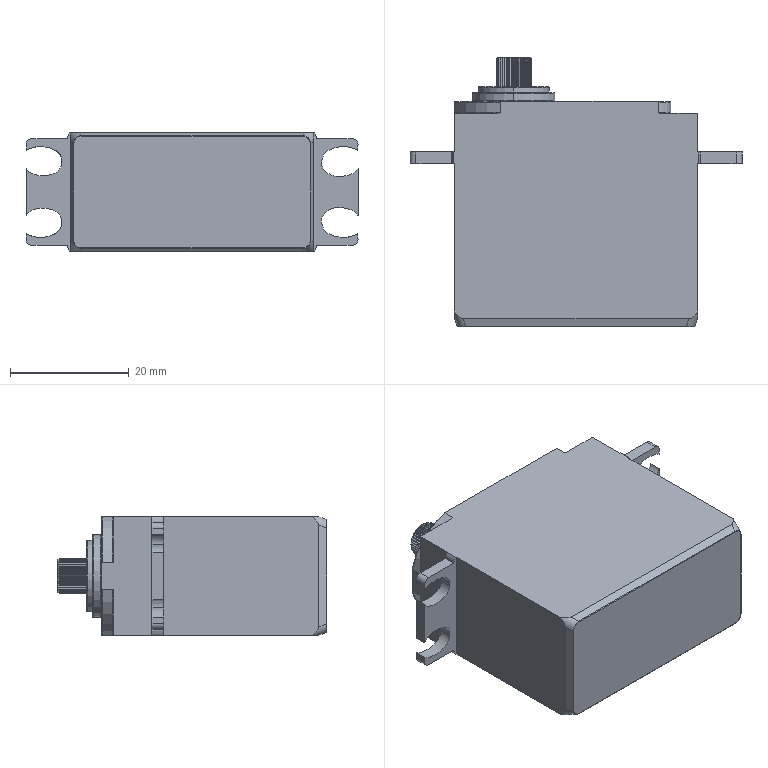Part | SolidWorks | features Cut 2, BaseBody 1 | 1 solid | 275 faces | box 56 x 45.5 x 20 mm | volume 31577 mm3 | plane 117 | cylinder 80 | cone 40 | torus 20 | spline 18 | commonest cylinder face diameters 0.1 x51 3 x10 0.2 x8 2 x4 12 x2 14 x2